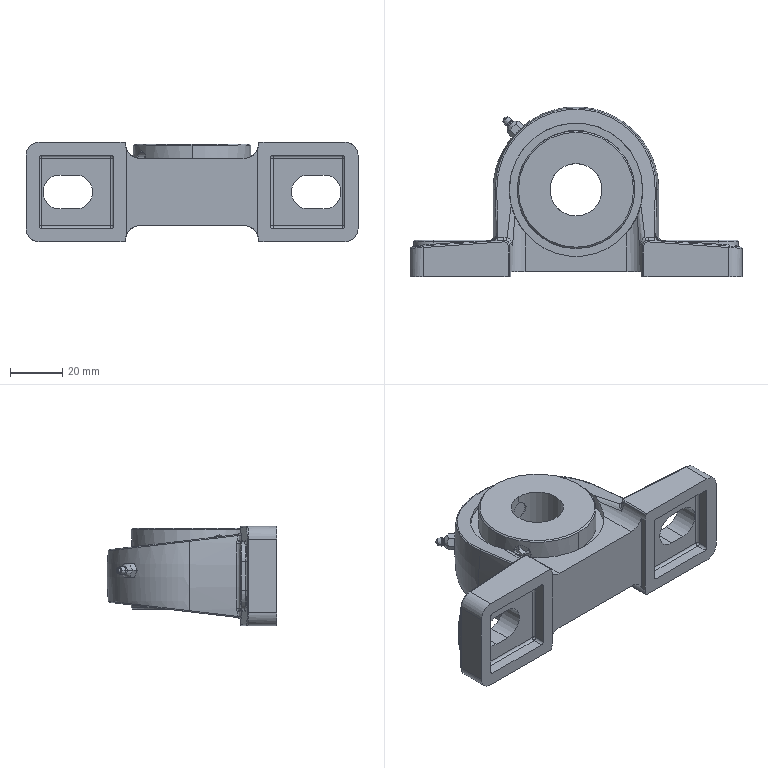Part | SolidWorks | features BaseBody 1 | 1 solid | 243 faces | box 127 x 65 x 38 mm | volume 109407 mm3 | cylinder 79 | plane 70 | spline 58 | cone 14 | torus 12 | sphere 10 | commonest cylinder face diameters 1 x22 2 x16 6.667 x9 3 x4 10 x4 12 x4